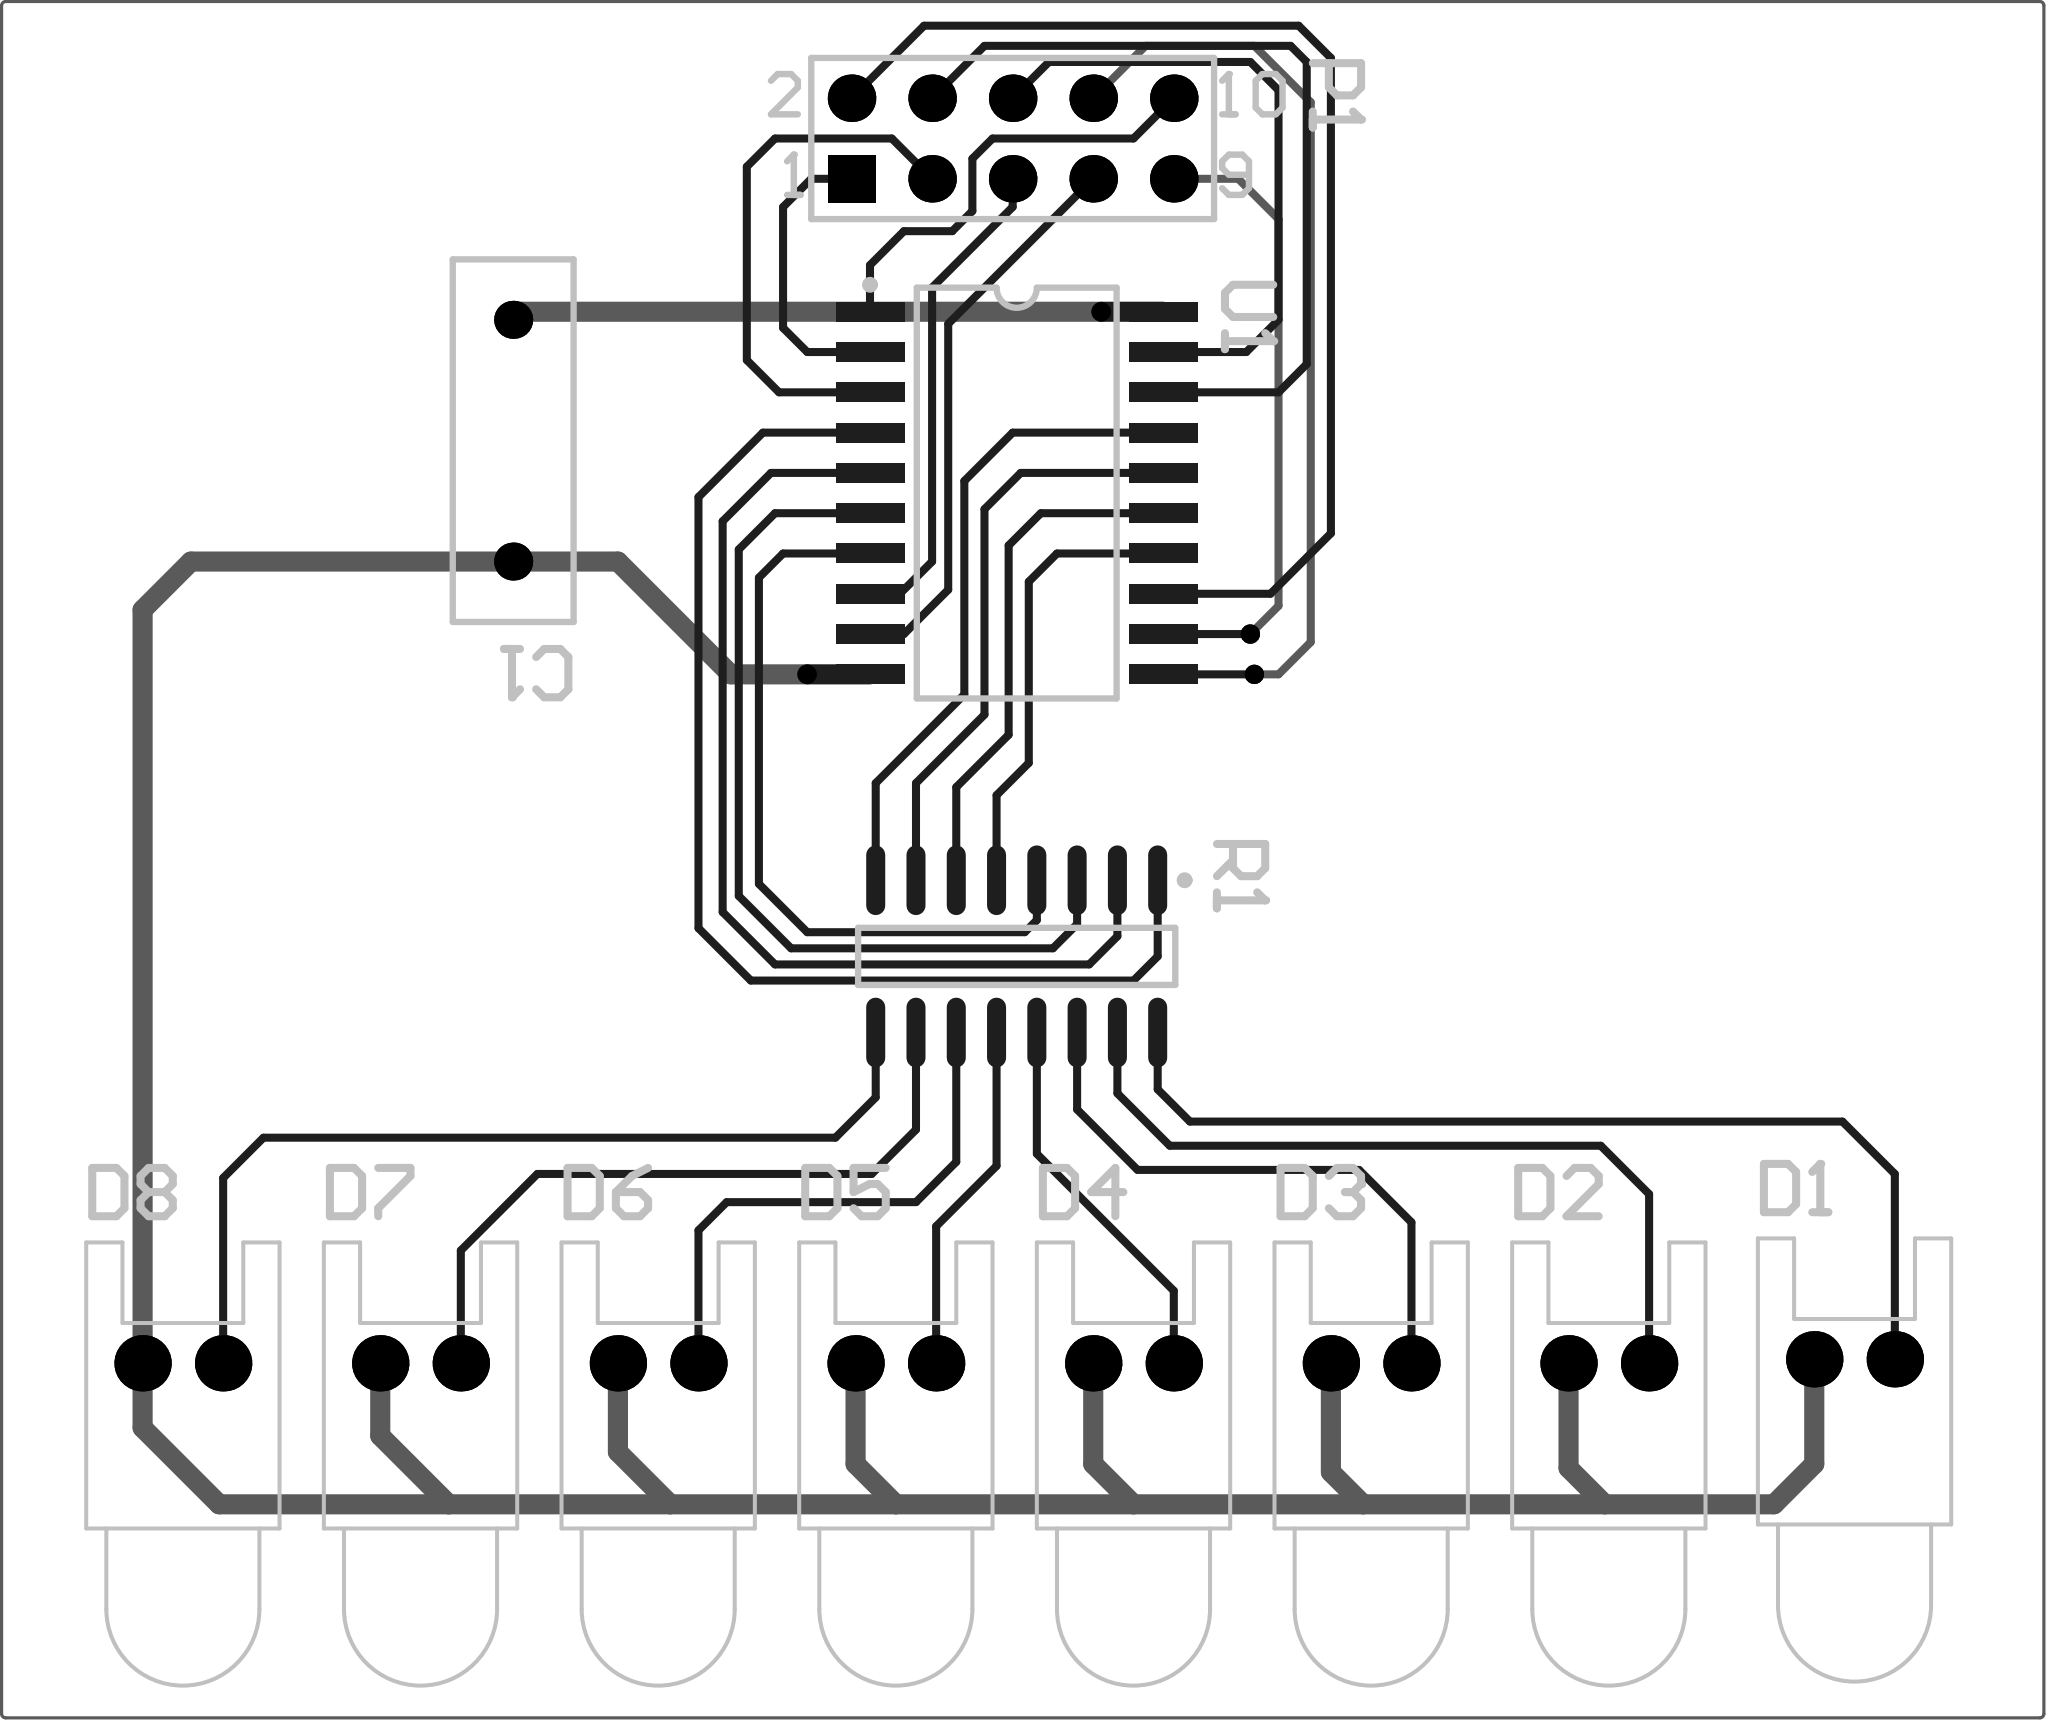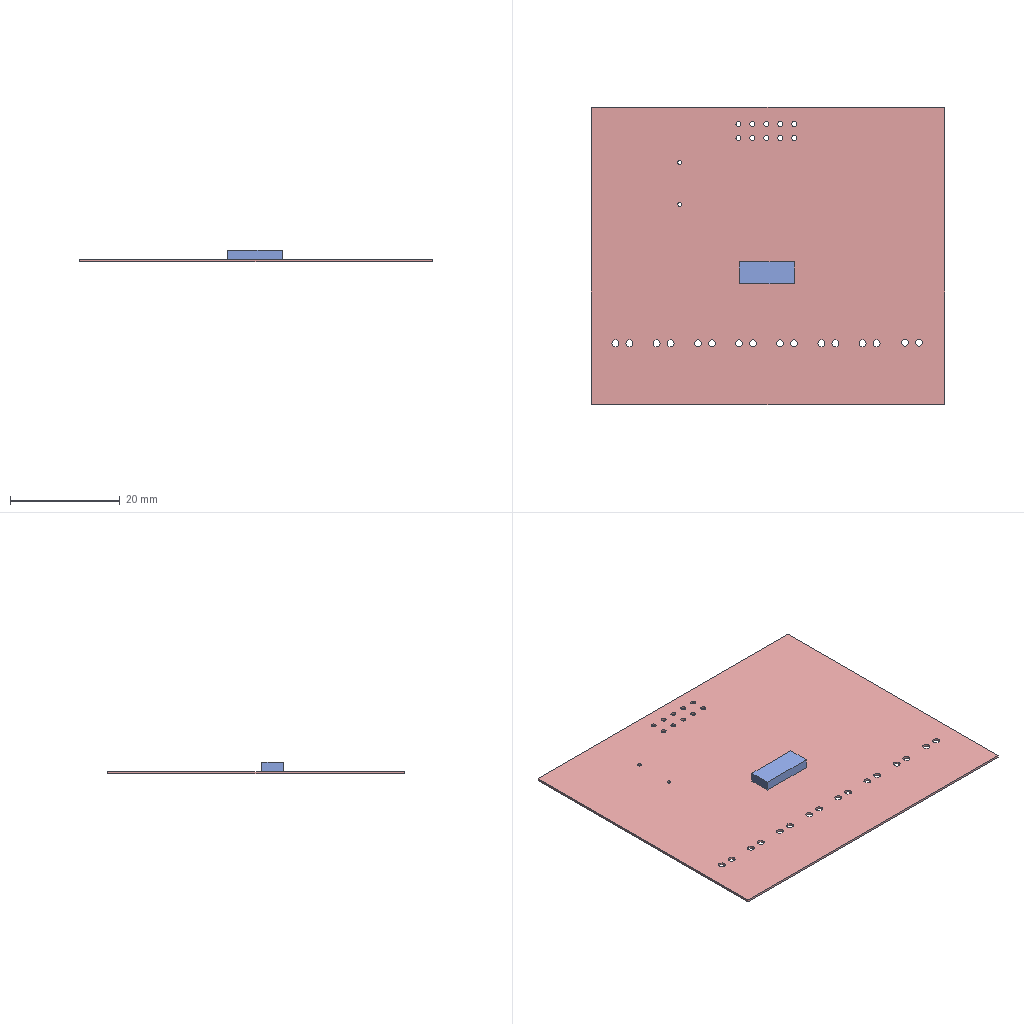Circuit board layout | Altium Designer | box 64.4 x 54.1 x 2.2 mm
Layer stack:
# Altium Designer layer stack of  (unit mm; dielectric type: 0 none, 1 core, 2 prepreg, 3 surface material)
index,name,kind,layer,copper_thickness_mm,dielectric_type,dielectric_thickness_mm,dielectric_material,dielectric_constant
0,Top Paste,other,,,,,,
1,Top Overlay,other,,,,,,
2,Top Solder,dielectric,,,3,0.0102,Solder Resist,3.5
3,Top Layer,copper,Top Layer,0.0356,,,,
4,Dielectric 1,dielectric,,,0,0.32,FR-4,4.8
5,Bottom Layer,copper,Bottom Layer,0.0356,,,,
6,Bottom Solder,dielectric,,,3,0.0102,Solder Resist,3.5
7,Bottom Overlay,other,,,,,,
8,Bottom Paste,other,,,,,,
# drill layer pairs: low layer,high layer
drill_pair,Top Layer,Bottom Layer
Part placement:
Designator,Comment,Layer,Footprint,Center-X(mm),Center-Y(mm),Rotation
U1,TPIC6B273DW,TopLayer,DW020,90.932,81.153,270
R1,Res Pack3,TopLayer,SO-16_N,90.932,66.548,270
P1,Header 5X2,TopLayer,HDR2X5,90.805,92.329,360
D8,LED0,TopLayer,LED-0,64.643,53.721,0
D7,LED0,TopLayer,LED-0,72.136,53.721,0
D6,LED0,TopLayer,LED-0,79.629,53.721,0
D5,LED0,TopLayer,LED-0,87.122,53.721,0
D4,LED0,TopLayer,LED-0,94.615,53.721,0
D3,LED0,TopLayer,LED-0,102.108,53.721,0
D2,LED0,TopLayer,LED-0,109.601,53.721,0
D1,LED0,TopLayer,LED-0,117.348,53.848,0
C1,Cap,TopLayer,RAD-0.3,75.057,82.804,270
Pad and via stacks:
# Altium Designer via and pad stacks of  (unit mm). Each distinct definition once, with the count of objects using it.
# via: kind,start_layer,end_layer,hole_mm,diameter_mm,mode(0 simple;1 top-mid-bottom;2 full stack),diameter_per_layer,count,example_net
# pad: kind,layer,hole_mm,hole_type(0 round;1 square;2 slot),plating,top_size,top_shape(1 round;2 rect;3 octagon;9 rounded rect),mid_size,bottom_size,mode,footprint,size_per_layer,count,example
pad,Multi-Layer,0.7,0,plated,1.2x1.2,1,1.2x1.2,1.2x1.2,0,RAD-0.3,,2,C1.2
pad,Multi-Layer,1.27,0,plated,1.778x1.778,1,1.778x1.778,1.778x1.778,0,LED-0,,16,D1.1
pad,Multi-Layer,0.9,0,plated,1.5x1.5,1,1.5x1.5,1.5x1.5,0,HDR2X5,,9,P1.10
pad,Multi-Layer,0.9,0,plated,1.5x1.5,2,1.5x1.5,1.5x1.5,0,HDR2X5,,1,P1.1
pad,Top Layer,0,0,plated,2.15x0.6,2,2.15x0.6,2.15x0.6,0,DW020,,20,U1.1
pad,Top Layer,0,0,plated,0.6x2.2,1,0.6x2.2,0.6x2.2,0,SO-16_N,,16,R1.1
via,Top Layer,Bottom Layer,0.3048,0.6096,0,,4,GND
Design rules, without the lines most boards share:
# Altium Designer design rules of  (exported by Altium Designer, unit mm)
# columns: name | kind | enabled | priority | scope1 | scope2 | descriptor | typed fields (field=value)
SilkToSilkClearance | 55 | enabled | 1 | All | All | Silk to Silk (Clearance=0mil) (All),(All) |
SilkToSolderMaskClearance | 54 | enabled | 1 | IsPad | All | Silk To Solder Mask (Clearance=0mil) (IsPad),(All) |
MinimumSolderMaskSliver | 53 | enabled | 1 | All | All | Minimum Solder Mask Sliver (Gap=0mil) (All),(All) |
HoleToHoleClearance | 52 | enabled | 1 | All | All | Hole To Hole Clearance (Gap=10mil) (All),(All) | gap=0.254
DiffPairsRouting | 51 | enabled | 1 | All | All | Differential Pairs Uncoupled Length using the Gap Constraints (Min=10mil) (Max=10mil) (Prefered=10mil)  and Width Constraints (Min=15mil) (Max=15mil) (Prefered=15mil) (All) |
SolderMaskExpansion | 13 | enabled | 1 | All | All | Solder Mask Expansion (Expansion =4mil) (All) | expansion=0.1016
PasteMaskExpansion | 14 | enabled | 1 | All | All | Paste Mask Expansion (Expansion =0mil) (All) | expansion=0
RoutingVias | 11 | enabled | 1 | All | All | Routing Via (MinHoleWidth=28mil) (MaxHoleWidth=28mil) (PreferredHoleWidth=28mil) (MinWidth=50mil) (MaxWidth=50mil) (PreferedWidth=50mil) (All) | via_min_hole=0.7112 via_max_hole=0.7112 via_preferred_diameter=1.27 via_preferred_hole=0.7112
Width | 2 | enabled | 1 | All | All | Width Constraint (Min=10mil) (Max=30mil) (Preferred=10mil) (All) |
PolygonConnect | 20 | enabled | 1 | All | All | Polygon Connect Rule(Relief Connect )(Conductor Width=10mil) (Relief Angle=90 Angle) (Entries=4) (Air Gap Width=10mil) (All),(All) | connect_style(0=relief,1=direct,2=none)=0 relief_conductor_width=0.254 relief_entries=4
PlaneConnect | 6 | enabled | 1 | All | All | Power Plane Connect Rule(Relief Connect )(Expansion=20mil) (Conductor Width=10mil) (Air Gap=10mil) (Entries=4) (All) | relief_conductor_width=0.254 relief_entries=4 relief_expansion=0.508
Clearance | 0 | enabled | 1 | All | All | Clearance Constraint (Gap=10mil) (All),(All) | gap=0.254
Classes set for this board:
# Altium Designer classes of  (member kind: 0 net, 1 component, 2 from-to, 3 pad, 4 layer, 5 differential pair, 6 design channel, 7 polygon, 8 structure, 9 xSignal)
# columns: class name | member kind | superclass | members
Sheet1 | 1 | no | C1; D1; D2; D3; D4; D5; D6; D7; D8; P1; R1; U1;